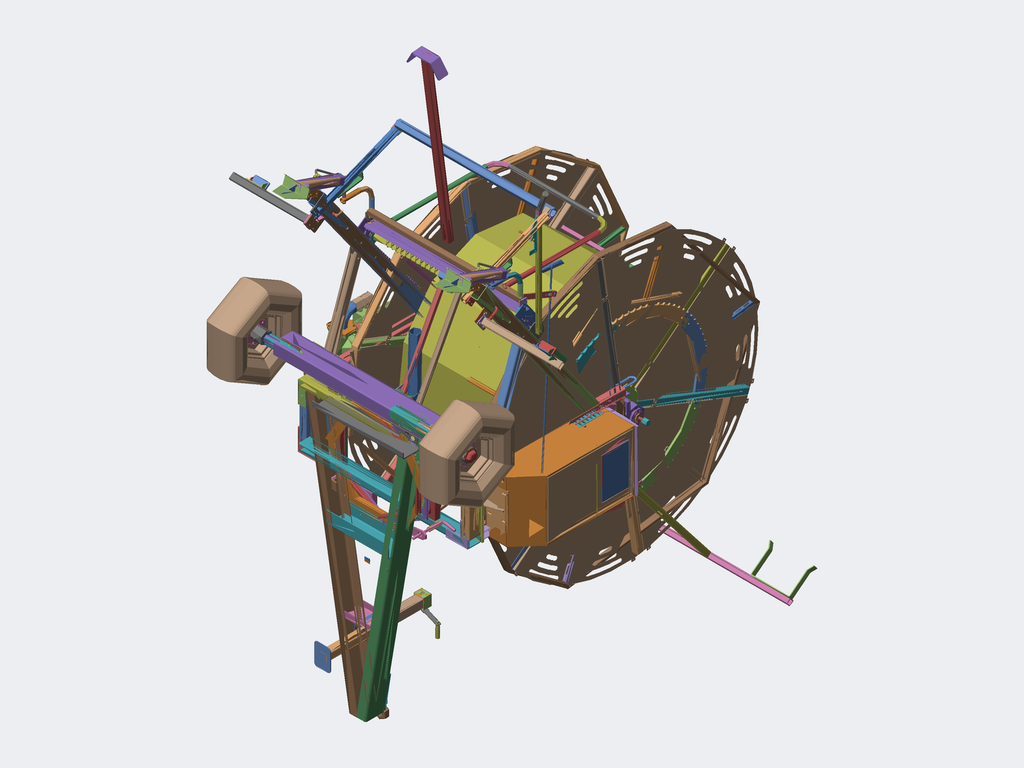Assembly | SolidWorks | 198 different items | 556 placed
Parts list (item | name | quantity | parent item | size | volume | features):
1 | 08B Inner Chain Link | x1 | - | - | - | -
2 | (subassembly) | x1 | - | - | - | features CompositeCurve 2
3 | (subassembly) | x1 | - | - | 42347469 mm3 | features CompositeCurve 25, ReferencePattern 11, InContextFeatHolder 2, MirrorCompFeat 2, LocalCirPattern 1
4 | (subassembly) | x1 | - | 1275 x 1167 x 393.469 mm | 1515109 mm3 | features CompositeCurve 9, ReferencePattern 5, MirrorCompFeat 1
5 | (subassembly) | x1 | - | - | - | features CompositeCurve 14
6 | (subassembly) | x1 | - | 850 x 850 x 62 mm | 6412042 mm3 | features ReferencePattern 139, CompositeCurve 9, LocalCirPattern 1
7 | (subassembly) | x1 | - | 138 x 180 x 325 mm | 523357 mm3 | features CompositeCurve 2
8 | (subassembly) | x1 | - | 105 x 440 x 68.5 mm | 381290 mm3 | features CompositeCurve 20
9 | (subassembly) | x2 | - | - | - | features CompositeCurve 6
10 | (subassembly) | x1 | - | - | - | features CompositeCurve 5
11 | (subassembly) | x2 | - | 84 x 93.542 x 20.19 mm | 15903 mm3 | features CompositeCurve 1
12 | (subassembly) | x1 | - | 1209 x 993.396 x 13.92 mm | 70663 mm3 | features ReferencePattern 244, LocalChainPattern 1
13 | (subassembly) | x1 | - | - | - | -
14 | (subassembly) | x2 | in 20 | 35 x 6.3 x 40 mm | 3119 mm3 | -
15 | (subassembly) | x1 | in 20 | 82.44 x 15.115 x 33.039 mm | 9980 mm3 | features CompositeCurve 1
16 | (subassembly) | x1 | - | 390 x 227.837 x 82 mm | 1530239 mm3 | -
17 | (subassembly) | x1 | - | 520 x 920 x 319.997 mm | 6570455 mm3 | features InContextFeatHolder 2
18 | (subassembly) | x1 | - | 550.016 x 318.498 x 397.435 mm | 1409303 mm3 | features CompositeCurve 37
19 | (subassembly) | x2 | in 17 | 48.002 x 12.05 x 47 mm | 11187 mm3 | features AEMSimFeature 1
20 | (subassembly) | x1 | - | 1370 x 197 x 2359 mm | 12525634 mm3 | features InContextFeatHolder 8, CompositeCurve 2
21 | (subassembly) | x1 | - | 1625 x 1990 x 1408 mm | 21000923 mm3 | features CompositeCurve 16
22 | (subassembly) | x1 | - | 51.4 x 48 x 1470 mm | 137893 mm3 | features CompositeCurve 3
23 | (subassembly) | x2 | - | 710 x 710 x 743.5 mm | 77284937 mm3 | features CompositeCurve 25, Cut 1
24 | (subassembly) | x1 | - | 335.143 x 891.073 x 1473 mm | 5779817 mm3 | features CompositeCurve 45, InContextFeatHolder 1
25 | (subassembly) | x1 | in 24 | 48 x 51.5 x 108 mm | 78961 mm3 | features CompositeCurve 3
26 | - | x1 | in 18 | 140 x 105.523 x 353.223 mm | 225582 mm3 | features BaseBody 9
27 | - | x1 | in 4 | 1275 x 1167 x 350.869 mm | 1494130 mm3 | features ICE 4, Fillet 2, WeldCornerFeat 2, WeldMemberFeat 2, 3DProfileFeature 1, MirrorSolid 1, WeldmentFeature 1
28 | - | x1 | in 22 | 1440 x 10 x 10 mm | 113097 mm3 | features Revolution 1
29 | - | x1 | in 6 | 850 x 850 x 48 mm | 3078442 mm3 | features Cut 1, Extrusion 1, HoleWzd 1, ICE 1, SweepCut 1
30 | - | x1 | in 6 | 850 x 850 x 48 mm | 3032308 mm3 | features ICE 2, Extrusion 1, SweepCut 1
31 | - | x140 | in 6 | 16 x 16 x 16 mm | 2145 mm3 | features Revolution 1
32 | - | x2 | in 9 | 17.852 x 45 x 36.623 mm | 5887 mm3 | features Bending 1, FlatPattern 1, SMBaseFlange 1, SheetMetal 1
33 | - | x1 | - | 87.114 x 117.396 x 10 mm | 59196 mm3 | features Extrusion 1
34 | - | x2 | in 9 | 505 x 200 x 74.971 mm | 438985 mm3 | features ICE 3, EdgeFlange 2, FlatPattern 1, Gusset 1, SMBaseFlange 1, SheetMetal 1, SweepThread 1, WeldMemberFeat 1, WeldmentFeature 1
35 | - | x2 | - | 127.5 x 127.5 x 15 mm | 40689 mm3 | features ICE 1, Sweep 1
36 | - | x1 | in 2 | 81.4 x 88.4 x 66.2 mm | 32314 mm3 | features ICE 3, CornerFeat 1, EdgeFlange 1, Fillet 1, FlatPattern 1, SMBaseFlange 1, SheetMetal 1
37 | - | x2 | in 9 | 390 x 100 x 60 mm | 365741 mm3 | features ICE 3, HoleWzd 1, MirrorSolid 1, WeldMemberFeat 1, WeldmentFeature 1
38 | - | x1 | - | 137.972 x 180 x 185 mm | 377579 mm3 | features Chamfer 1, ICE 1, Revolution 1
39 | - | x1 | - | 180 x 400 x 115 mm | 1229288 mm3 | features ICE 4, Fillet 3, Gusset 2, Extrusion 1, HoleWzd 1
40 | - | x1 | in 7 | 137.972 x 180 x 185 mm | 377579 mm3 | features Chamfer 1, ICE 1, MoveCopyBody 1, Revolution 1
41 | - | x1 | in 2 | 565 x 115 x 75 mm | 595954 mm3 | features ICE 3, WeldMemberFeat 2, EdgeFlange 1, FlatPattern 1, SMBaseFlange 1, SheetMetal 1, WeldmentFeature 1
42 | - | x1 | in 10 | 180 x 60 x 10 mm | 103818 mm3 | features Extrusion 1
43 | - | x1 | in 17 | 55 x 19.5 x 39.375 mm | 9114 mm3 | features ICE 11, Fillet 7, BossThin 2, CutThin 2, LPattern 2, CirPattern 1, Emboss 1, Extrusion 1, MirrorPattern 1, Scale 1
44 | - | x1 | in 10 | 60 x 116.5 x 60 mm | 137866 mm3 | features ICE 3, Fillet 1, Revolution 1
45 | - | x1 | in 10 | 30 x 190 x 28 mm | 58353 mm3 | features Chamfer 1, ICE 1, Revolution 1
46 | - | x2 | in 10 | 14 x 47 x 47 mm | 15915 mm3 | features Revolution 1
47 | - | x1 | in 2 | 5 x 5 x 23 mm | 451.339 mm3 | features Extrusion 1, Fillet 1
48 | - | x1 | in 20 | 604.658 x 439.557 x 2 mm | 390296 mm3 | features Extrusion 1, ICE 1
49 | - | x2 | - | 310 x 184.907 x 93.1 mm | 1419775 mm3 | features ICE 13, Fillet 12, Draft 4, RevCut 2, Revolution 2, 3DProfileFeature 1, Chamfer 1, CirPattern 1, HoleWzd 1, RefAxis 1
50 | - | x2 | in 8 | 52 x 7.4 x 3.7 mm | 537.554 mm3 | features ICE 1, Sweep 1
51 | - | x2 | in 23 | 64 x 9.2 x 4.6 mm | 1032 mm3 | features ICE 1, Sweep 1
52 | - | x1 | in 8 | 40 x 440 x 14 mm | 235600 mm3 | features Extrusion 1, ICE 1
53 | - | x1 | in 8 | 105 x 40 x 40 mm | 52528 mm3 | features HoleWzd 1, ICE 1, WeldMemberFeat 1, WeldmentFeature 1
54 | - | x1 | - | 120.458 x 120.458 x 175 mm | 185173 mm3 | features Chamfer 2, Extrusion 1, ICE 1, LPattern 1, Revolution 1
55 | - | x2 | in 11 | 84 x 93.542 x 20 mm | 12226 mm3 | features ICE 3, Extrusion 1
56 | - | x2 | in 11 | 9 x 9 x 20 mm | 1148 mm3 | features 3DProfileFeature 1, Extrusion 1, HoleWzd 1
57 | - | x2 | in 11 | 17.5 x 9 x 20 mm | 1066 mm3 | features ICE 2, Extrusion 1
58 | - | x1 | - | 81 x 81 x 40.5 mm | 121304 mm3 | features RevCut 2, MoveCopyBody 1, Sweep 1, SweepCut 1
59 | - | x1 | - | - | - | features 3DProfileFeature 4, Helix 1, SweepRefSurface 1
60 | - | x1 | - | 39.501 x 141.742 x 39.499 mm | 29526 mm3 | features 3DProfileFeature 2, Helix 1, Sweep 1
61 | - | x1 | - | 1433 x 80 x 270.762 mm | 1230459 mm3 | features 3DProfileFeature 1, EdgeFlange 1, Fillet 1, FlatPattern 1, HoleWzd 1, SMBaseFlange 1, SheetMetal 1, WeldMemberFeat 1, WeldmentFeature 1
62 | - | x2 | in 10 | 46 x 46 x 1 mm | 1316 mm3 | features Extrusion 1
63 | - | x1 | in 10 | - | - | features ExtendRefSurface 10, ICE 9, OffsetRefSurface 8, TrimRefSurface 6, Fillet 4, ThickenCut 4, SewRefSurface 2, Split 2, Chamfer 1, Helix 1, MirrorPattern 1, Revolution 1, SweepCut 1
64 | - | x1 | in 10 | 418.512 x 837.703 x 220 mm | 967255 mm3 | features ICE 5, Chamfer 4, Extrusion 1, MirrorSolid 1, WeldMemberFeat 1, WeldmentFeature 1
65 | - | x2 | in 21 | 70 x 105 x 12 mm | 65059 mm3 | features Extrusion 1
66 | - | x1 | - | 1270 x 184.784 x 82.347 mm | 924037 mm3 | features ICE 3, SM3dBend 3, Fillet 1, FlatPattern 1, SMBaseFlange 1, SheetMetal 1
67 | - | x1 | in 20 | 25 x 35 x 32 mm | 4524 mm3 | features Extrusion 1, ICE 1
68 | - | x2 | in 9 | 208.199 x 56 x 66 mm | 34151 mm3 | features 3DProfileFeature 2, Sweep 1
69 | - | x1 | in 18 | 132.972 x 76 x 132.966 mm | 175775 mm3 | features Chamfer 1, ICE 1, Revolution 1
70 | - | x1 | in 17 | 520 x 920 x 319.997 mm | 6254954 mm3 | features EdgeFlange 13, ICE 11, FlatPattern 7, SheetMetal 6, SMBaseFlange 5, LPattern 3, Cut 2, Chamfer 1, FormToolInstance 1, MirrorSolid 1, SolidToSheetMetal 1
71 | - | x12 | in 3 | 1022 x 1094 x 15 mm | 731412 mm3 | features SMBaseFlange 8, EdgeFlange 6, ICE 2, BreakCorner 1, FlatPattern 1, SheetMetal 1
72 | - | x1 | - | 1086 x 1346 x 2725 mm | 2854762 mm3 | features 3DProfileFeature 2, FlatPattern 2, ICE 2, MirrorSolid 2, MoveCopyBody 2, Stock 2, MirrorPattern 1, SheetMetal 1, WeldMemberFeat 1, WeldmentFeature 1
73 | - | x1 | - | 2700 x 120 x 40 mm | 1184354 mm3 | features WeldMemberFeat 2, 3DProfileFeature 1, WeldCornerFeat 1, WeldmentFeature 1
74 | - | x1 | - | 115 x 120 x 648 mm | 459448 mm3 | features Gusset 4, Cut 1, Extrusion 1, Fillet 1, FlatPattern 1, ICE 1, SMBaseFlange 1, SheetMetal 1, WeldMemberFeat 1, WeldmentFeature 1
75 | - | x1 | in 25 | 40 x 47.5 x 59 mm | 50942 mm3 | features ICE 3, Extrusion 1, Fillet 1, HoleWzd 1
76 | - | x1 | in 18 | 96 x 70 x 96 mm | 39871 mm3 | features Revolution 1, Shell 1
77 | - | x1 | in 10 | 47 x 47 x 43 mm | 54544 mm3 | features Fillet 3, ICE 3, Chamfer 1, Extrusion 1, HoleWzd 1
78 | - | x1 | in 18 | 29 x 29 x 50 mm | 17318 mm3 | features Extrusion 1
79 | - | x1 | in 15 | 24.5 x 13 x 30 mm | 2874 mm3 | features Extrusion 1, ICE 1
80 | - | x1 | in 24 | 89.972 x 76 x 125.857 mm | 125660 mm3 | features Chamfer 1, Revolution 1, Split 1
81 | - | x1 | in 15 | 70.865 x 12.969 x 30 mm | 5794 mm3 | features ICE 2, Extrusion 1, Fillet 1
82 | - | x1 | in 15 | 11 x 33 x 11 mm | 1312 mm3 | features Revolution 1
83 | - | x1 | - | 158.16 x 158.6 x 7.2 mm | 83678 mm3 | features ICE 5, Revolution 5, CirPattern 3, LPattern 2
84 | - | x1 | in 8 | 88.261 x 91.8 x 14.2 mm | 61120 mm3 | features ICE 5, Revolution 5, CirPattern 3, LPattern 2
85 | - | x1 | in 16 | 227.837 x 280 x 82 mm | 957079 mm3 | features Extrusion 1, Fillet 1, HoleWzd 1, ICE 1
86 | - | x1 | in 16 | 45 x 100 x 290 mm | 523268 mm3 | features ICE 3, Extrusion 1, Fillet 1
87 | - | x1 | in 17 | 440 x 240 x 2 mm | 211121 mm3 | features Cut 1, Extrusion 1
88 | - | x1 | - | 32 x 32 x 55 mm | 17666 mm3 | features Extrusion 1
89 | - | x1 | in 25 | 15 x 15 x 45 mm | 5260 mm3 | features Chamfer 4, ICE 3, Extrusion 1
90 | - | x1 | in 25 | - | - | features ICE 15, RefSurface 4, Revolution 4, BaseBody 1, Chamfer 1
91 | - | x1 | in 24 | 132.972 x 76 x 132.966 mm | 179855 mm3 | features Chamfer 1, Revolution 1
92 | - | x2 | - | 55 x 40 x 210.02 mm | 80598 mm3 | features FlatPattern 1, SM3dBend 1, SMBaseFlange 1, SheetMetal 1
93 | - | x2 | in 2 | 30 x 30 x 8 mm | 2019 mm3 | features ICE 3, Extrusion 1
94 | - | x1 | in 24 | 76 x 76 x 525 mm | 638592 mm3 | features Chamfer 1, Extrusion 1
95 | - | x3 | in 7, 18 | 76 x 76 x 140 mm | 145605 mm3 | features Chamfer 2, Extrusion 1, ICE 1, LPattern 1
96 | - | x1 | in 18 | 75 x 130 x 10 mm | 89834 mm3 | features Extrusion 1
97 | - | x1 | in 21 | 85 x 80 x 10 mm | 64814 mm3 | features Extrusion 1, HoleWzd 1
98 | - | x1 | in 18 | 182 x 76.1 x 76.1 mm | 182460 mm3 | features Chamfer 1, WeldMemberFeat 1, WeldmentFeature 1
99 | - | x1 | in 18 | 211.75 x 403.566 x 147.274 mm | 1044578 mm3 | features MoveCopyBody 11, Stock 10, ICE 6, Chamfer 1, WeldMemberFeat 1, WeldmentFeature 1
100 | - | x1 | in 18 | 110 x 30 x 35 mm | 17166 mm3 | features FlatPattern 1, Jog 1, SMBaseFlange 1, SheetMetal 1
101 | - | x1 | in 18 | 120 x 120 x 80 mm | 384227 mm3 | features ICE 4, Chamfer 1, Extrusion 1
102 | - | x1 | in 18 | 132.972 x 76 x 132.966 mm | 179855 mm3 | features Chamfer 1, Revolution 1
103 | - | x1 | in 24 | 177 x 120 x 80 mm | 437085 mm3 | features ICE 5, Chamfer 3, Cut 1, Extrusion 1
104 | - | x1 | - | 87.114 x 117.396 x 10 mm | 59196 mm3 | features MirrorStock 1
105 | - | x1 | - | 115 x 120 x 648 mm | 459448 mm3 | features MirrorStock 1
106 | - | x1 | in 2 | 28 x 28 x 120.982 mm | 58497 mm3 | features MBimport 1
107 | - | x1 | - | 500 x 710.009 x 320 mm | 1088969 mm3 | features ICE 6, EdgeFlange 4, Fillet 3, Chamfer 2, SMBaseFlange 2, SheetMetal 2, Cut 1, FlatPattern 1, Shell 1
108 | - | x2 | in 19 | 29.75 x 12.05 x 47 mm | 4659 mm3 | features BaseBody 1
109 | - | x2 | in 19 | 29.75 x 12.05 x 47 mm | 6528 mm3 | features BaseBody 1
110 | - | x123 | in 12 | 24.41 x 13.399 x 13.92 mm | 574.494 mm3 | features Boss 2, DeleteBody 1, Extrusion 1, MirrorSolid 1
111 | - | x3 | in 6, 23 | 12.702 x 18 x 11 mm | 1039 mm3 | features ICE 9, Revolution 9, Fillet 2
112 | - | x1 | in 22 | 55 x 48 x 24 mm | 13448 mm3 | features ICE 4, Fillet 2, Revolution 2, Chamfer 1, MirrorSolid 1, RevCut 1, Sweep 1
113 | - | x2 | in 9 | 47.841 x 25 x 47.841 mm | 21610 mm3 | features BaseBody 1
114 | - | x1 | in 10 | 20 x 8 x 7 mm | 1023 mm3 | features Extrusion 1, Fillet 1
115 | - | x2 | in 21 | 12 x 47 x 47 mm | 11391 mm3 | features Revolution 5, CirPattern 2, RefAxis 1, RevCut 1
116 | - | x4 | in 23 | 18 x 80 x 80 mm | 53386 mm3 | features Revolution 5, CirPattern 2, RefAxis 1, RevCut 1
117 | - | x1 | in 21 | 10.9 x 9.44 x 6.4 mm | 370.095 mm3 | features Cut 2, Chamfer 1, Extrusion 1
118 | - | x1 | in 21 | 16 x 11.547 x 10 mm | 685.126 mm3 | features Chamfer 2, RevCut 2, Revolution 2, Extrusion 1, ICE 1
119 | - | x2 | in 10 | 86.4 x 18.475 x 16 mm | 7671 mm3 | features RevCut 3, Extrusion 1, Fillet 1, LPattern 1, Revolution 1
120 | - | x3 | in 22 | 31.4 x 18.475 x 16 mm | 3338 mm3 | features RevCut 3, Extrusion 1, Fillet 1, LPattern 1, Revolution 1
121 | - | x1 | in 17 | - | 5761098 mm3 | features BaseBody 28
122 | - | x2 | in 11 | 44 x 11.547 x 10 mm | 1463 mm3 | features RevCut 3, Extrusion 1, Fillet 1, LPattern 1, Revolution 1
123 | - | x1 | - | 127.5 x 20.785 x 18 mm | 15623 mm3 | features RevCut 3, Extrusion 1, Fillet 1, LPattern 1, Revolution 1
124 | - | x6 | in 4 | 18 x 20.785 x 10.8 mm | 2151 mm3 | features Cut 2, Extrusion 1
125 | - | x6 | in 10, 20 | 24 x 27.713 x 14.8 mm | 5128 mm3 | features Cut 2, Extrusion 1
126 | - | x7 | in 10, 22 | 16 x 18.475 x 8.4 mm | 1366 mm3 | features ICE 2, RevCut 2, Extrusion 1
127 | - | x1 | - | 18 x 20.785 x 10.8 mm | 2103 mm3 | features Cut 2, Chamfer 1, Extrusion 1
128 | - | x1 | in 16 | 52.646 x 60.79 x 34.7 mm | 49893 mm3 | features Cut 3, Chamfer 1, CirPattern 1, Extrusion 1
129 | - | x2 | in 2 | 25.6 x 29.56 x 17 mm | 6436 mm3 | features Cut 2, Chamfer 1, Extrusion 1
130 | - | x2 | in 4 | 18 x 20.785 x 21 mm | 4036 mm3 | features Cut 3, Extrusion 1, Revolution 1
131 | - | x2 | in 10 | 16.182 x 16.166 x 2 mm | 241.9 mm3 | features Extrusion 1
132 | - | x1 | in 2 | 35 x 35 x 19 mm | 13347 mm3 | features ICE 4, Blend 1, Chamfer 1, Extrusion 1
133 | - | x1 | in 10 | 25.172 x 25.146 x 3.2 mm | 909.871 mm3 | features Extrusion 1
134 | - | x2 | in 23 | 85.5 x 83.408 x 2.5 mm | 3180 mm3 | features Extrusion 1
135 | - | x1 | in 10 | 50.5 x 48.578 x 1.5 mm | 759.16 mm3 | features Extrusion 1
136 | - | x2 | in 23 | 36.439 x 36.377 x 6 mm | 3321 mm3 | features Extrusion 1
137 | - | x2 | in 23 | 34.251 x 39.55 x 23.9 mm | 13268 mm3 | features Cut 3, Chamfer 1, CirPattern 1, Extrusion 1
138 | - | x2 | in 10 | 20 x 20 x 2 mm | 455.138 mm3 | features Extrusion 1
139 | - | x5 | in 2, 9 | 24 x 24 x 2.5 mm | 799.143 mm3 | features Extrusion 1
140 | - | x4 | in 8, 10 | 30 x 30 x 3 mm | 1440 mm3 | features Extrusion 1
141 | - | x2 | in 10 | 37 x 37 x 3 mm | 2187 mm3 | features Extrusion 1
142 | - | x2 | in 23 | 44 x 44 x 4 mm | 4119 mm3 | features Extrusion 1
143 | - | x1 | in 3 | 14.048 x 1371 x 1371 mm | 4173248 mm3 | features CirPattern 2, ICE 2, Cut 1, HoleWzd 1, Revolution 1
144 | - | x2 | in 9 | 11 x 18.425 x 12.702 mm | 861.691 mm3 | features BaseBody 1
145 | - | x1 | in 17 | 110 x 39 x 78.75 mm | 72913 mm3 | features ICE 11, Fillet 7, BossThin 2, CutThin 2, LPattern 2, CirPattern 1, Emboss 1, Extrusion 1, MirrorPattern 1
146 | - | x1 | - | - | - | features Sweep 6, Helix 5, 3DProfileFeature 2
147 | - | x1 | - | 379.2 x 630 x 367.794 mm | 25839555 mm3 | features ICE 35, CirPattern 5, Revolution 5, Fillet 3, Blend 2, Chamfer 2, CombineBodies 2, MirrorPattern 1, MirrorSolid 1, MoveFace 1, Scale 1
148 | - | x1 | in 20 | 1370 x 90 x 169.999 mm | 3268075 mm3 | features Cut 2, WeldMemberFeat 2, FlatPattern 1, MirrorSolid 1, SM3dBend 1, SMBaseFlange 1, SheetMetal 1, WeldmentFeature 1
149 | - | x1 | in 20 | 2311 x 160 x 74.999 mm | 3368982 mm3 | features Split 4, Cut 2, 3DProfileFeature 1, FlatPattern 1, Fold 1, HoleWzd 1, SM3dBend 1, SMBaseFlange 1, SheetMetal 1, UnFold 1, WeldmentFeature 1
150 | - | x1 | in 20 | 92 x 68.996 x 44.996 mm | 49140 mm3 | features Fillet 1, FlatPattern 1, SM3dBend 1, SMBaseFlange 1, SheetMetal 1
151 | - | x1 | in 20 | 2311 x 160 x 74.999 mm | 3368985 mm3 | features Split 4, Cut 2, 3DProfileFeature 1, FlatPattern 1, Fold 1, HoleWzd 1, SM3dBend 1, SMBaseFlange 1, SheetMetal 1, UnFold 1, WeldmentFeature 1
152 | - | x1 | in 20 | 750 x 155 x 194.999 mm | 1173169 mm3 | features Cut 1, FlatPattern 1, HoleWzd 1, SM3dBend 1, SMBaseFlange 1, SheetMetal 1, Split 1
153 | - | x1 | in 20 | 300 x 155 x 54.999 mm | 345967 mm3 | features Split 2, FlatPattern 1, HoleWzd 1, SM3dBend 1, SMBaseFlange 1, SheetMetal 1
154 | - | x1 | in 8 | 20 x 58.5 x 20 mm | 12679 mm3 | features Chamfer 1, ICE 1, Revolution 1
155 | - | x1 | in 20 | 510 x 155 x 99.999 mm | 817688 mm3 | features FlatPattern 1, HoleWzd 1, ICE 1, SM3dBend 1, SMBaseFlange 1, SheetMetal 1, Split 1
156 | - | x1 | in 21 | 800 x 480 x 1.5 mm | 561110 mm3 | features FlatPattern 1, ICE 1, SMBaseFlange 1, SheetMetal 1
157 | - | x1 | in 21 | 1815 x 180 x 1367 mm | 6438478 mm3 | features ICE 12, Cut 6, WeldCornerFeat 5, WeldMemberFeat 5, 3DProfileFeature 3, Gusset 3, HoleWzd 3, DeleteBody 2, MirrorSolid 2, MoveCopyBody 2, Extrusion 1, Fillet 1, FlatPattern 1, SM3dBend 1, SMBaseFlange 1, SheetMetal 1, Sweep 1, WeldmentFeature 1
158 | - | x1 | in 21 | 1815 x 315 x 1367 mm | 6905440 mm3 | features ICE 15, Cut 6, WeldCornerFeat 4, WeldMemberFeat 4, 3DProfileFeature 3, Gusset 3, HoleWzd 3, Sweep 2, Extrusion 1, Fillet 1, FlatPattern 1, MirrorSolid 1, MoveCopyBody 1, SM3dBend 1, SMBaseFlange 1, SheetMetal 1, WeldmentFeature 1
159 | - | x2 | - | 1550 x 90 x 50 mm | 1146938 mm3 | features HoleWzd 2, LPattern 1, Split 1, WeldMemberFeat 1, WeldmentFeature 1
160 | - | x1 | - | 1030 x 86.429 x 90 mm | 351764 mm3 | features HoleWzd 2, ICE 1, WeldMemberFeat 1, WeldmentFeature 1
161 | - | x1 | in 3 | 2340 x 2340 x 60 mm | 8212314 mm3 | features WeldMemberFeat 3, ICE 2, 3DProfileFeature 1, Cut 1, WeldmentFeature 1
162 | - | x1 | in 3 | 2340 x 2340 x 85 mm | 8494790 mm3 | features FlatPattern 6, ICE 5, WeldMemberFeat 3, CirPattern 2, HoleWzd 2, 3DProfileFeature 1, EdgeFlange 1, Fillet 1, SMBaseFlange 1, SheetMetal 1, WeldmentFeature 1
163 | - | x1 | - | 1280 x 800 x 70.292 mm | 1562390 mm3 | features 3DProfileFeature 2, HoleWzd 2, ICE 2, MirrorSolid 2, WeldMemberFeat 2, WeldmentFeature 1
164 | - | x1 | in 8 | 20 x 68.5 x 20 mm | 13969 mm3 | features ICE 1, Revolution 1
165 | - | x1 | in 21 | 1400 x 880 x 118 mm | 7030026 mm3 | features ICE 4, HoleWzd 2, WeldMemberFeat 2, LPattern 1, MoveCopyBody 1, WeldmentFeature 1
166 | - | x1 | in 2 | - | - | features ICE 2, Chamfer 1, Extrusion 1, Helix 1, SweepCut 1
167 | - | x1 | - | 93.66 x 68.58 x 50.292 mm | 77419 mm3 | features ICE 4, ConnectionPoint 2, Fillet 2, MoveFace 2, Revolution 2, MoveCopyBody 1, RoutePoint 1, Scale 1
168 | - | x1 | in 18 | 100 x 140 x 44 mm | 86746 mm3 | features ICE 6, Fillet 2, Chamfer 1, Extrusion 1, MirrorPattern 1, Revolution 1
169 | - | x1 | in 2 | 110 x 200 x 40 mm | 43181 mm3 | features ICE 2, Fillet 1, Sweep 1
170 | - | x2 | in 14 | 20.65 x 6.3 x 40 mm | 1684 mm3 | features BaseBody 1
171 | - | x2 | in 14 | 20.65 x 6.3 x 40 mm | 1435 mm3 | features BaseBody 1
172 | - | x2 | in 9 | - | - | features ICE 2, Chamfer 1, Extrusion 1, Helix 1, SweepCut 1
173 | - | x1 | in 22 | 16 x 16 x 60 mm | 5278 mm3 | features Extrusion 1
174 | - | x2 | - | 110 x 260 x 20 mm | 106750 mm3 | features Chamfer 2, Sweep 1
175 | - | x1 | in 2 | 43.5 x 43.5 x 20 mm | 21997 mm3 | features ICE 2, Blend 1, Extrusion 1
176 | - | x2 | in 23 | 264 x 710 x 710 mm | 75274226 mm3 | features Revolution 2, ICE 1
177 | - | x2 | in 23 | 180 x 180 x 130 mm | 680348 mm3 | features ICE 7, HoleWzd 2, Chamfer 1, Extrusion 1
178 | - | x2 | in 23 | 495 x 60 x 60 mm | 418098 mm3 | features Cut 2, WeldMemberFeat 1, WeldmentFeature 1
179 | - | x2 | in 23 | 50 x 50 x 446 mm | 738051 mm3 | features ICE 2, Chamfer 1, Extrusion 1
180 | - | x2 | in 23 | 108 x 30 x 108 mm | 27953 mm3 | features ICE 1, Revolution 1
181 | - | x4 | in 18, 24 | 106 x 11.67 x 106 mm | 13391 mm3 | features Revolution 1
182 | - | x1 | in 24 | 76 x 184.67 x 76 mm | 170240 mm3 | features ICE 2, BlendCut 1, Revolution 1
183 | - | x1 | in 24 | 89 x 89 x 279.1 mm | 698533 mm3 | features Chamfer 2, ICE 2, Extrusion 1
184 | - | x1 | in 25 | 48 x 48 x 10 mm | 16281 mm3 | features Extrusion 1
185 | - | x1 | in 24 | 1176 x 89 x 89 mm | 3262124 mm3 | features ICE 5, 3DProfileFeature 2, Chamfer 2, Cut 1, DelFace 1, DeleteBody 1, HoleWzd 1, RefCurve 1, Revolution 1, Split 1, SurfCut 1
186 | - | x1 | - | - | - | features Fillet 1, MBimport 1
187 | - | x2 | in 23 | 5.21 x 79.5 x 79.5 mm | 14367 mm3 | features Chamfer 2, Revolution 1
188 | - | x1 | in 3 | 1520 x 1520 x 1030 mm | 12689787 mm3 | features WeldMemberFeat 2, CirPattern 1, Cut 1, FlatPattern 1, ICE 1, MirrorSolid 1, MoveCopyBody 1, SMBaseFlange 1, SheetMetal 1, WeldmentFeature 1
189 | - | x1 | in 2 | 30 x 30 x 7 mm | 2499 mm3 | features Extrusion 1, ICE 1
190 | - | x3 | in 2, 9 | 26 x 26 x 11.5 mm | 4545 mm3 | features Extrusion 1, Fillet 1
191 | - | x1 | - | 46.249 x 52.7 x 46.542 mm | 34114 mm3 | features ICE 3, Revolution 2
192 | - | x1 | in 2 | 498.5 x 130 x 180 mm | 585064 mm3 | features ICE 2, HoleWzd 1, WeldMemberFeat 1, WeldmentFeature 1
193 | - | x1 | in 24 | 89 x 89 x 95 mm | 239064 mm3 | features Chamfer 1, Extrusion 1, ICE 1
194 | - | x1 | - | 368.66 x 40 x 234.641 mm | 156675 mm3 | features EdgeFlange 2, FlatPattern 1, SMBaseFlange 1, SheetMetal 1
195 | - | x2 | - | 63 x 17.5 x 3 mm | 910.243 mm3 | features BaseBody 1, ICE 1, Scale 1
196 | - | x1 | - | 780 x 780 x 250 mm | 1146296 mm3 | features WeldCornerFeat 2, WeldMemberFeat 2, 3DProfileFeature 1, Cut 1, HoleWzd 1, MoveCopyBody 1, Split 1, WeldmentFeature 1
197 | - | x1 | in 10 | 88 x 88 x 25.063 mm | 77723 mm3 | features BaseBody 1
198 | GB/T 5786-2000[Hex Head Bolt Fine Thread Full Thread M12x1.5x90] | x1 | - | - | - | -
Mates (type | each side: item.copy, entity, surface, feature), first 400 of 510 lines:
In the top assembly
Width | 178.1 face plane Cold-formed Square Hollow Section gb/t6728-2002 60 X 60 X 4(1) | 178.1 face plane Cold-formed Square Hollow Section gb/t6728-2002 60 X 60 X 4(1) | 148.1 face plane Base-Flange 1 | assembly face
Width | 178.1 face plane Cold-formed Square Hollow Section gb/t6728-2002 60 X 60 X 4(1) | 178.1 face plane Cold-formed Square Hollow Section gb/t6728-2002 60 X 60 X 4(1) | assembly face | 148.1 face plane Base-Flange 1
Coincident | assembly face | 178.1 face
Width | 178.2 face plane Cold-formed Square Hollow Section gb/t6728-2002 60 X 60 X 4(1) | 178.2 face plane Cold-formed Square Hollow Section gb/t6728-2002 60 X 60 X 4(1) | assembly face | 148.1 face plane Base-Flange 1 | 2 times
Coincident | assembly face | 178.2 face
Concentric | 27.1 face cylinder Boss-Extrude 1 | 120.1 face cylinder Boss-Revolve 1
Coincident | 27.1 face plane Boss-Extrude 1 | 120.1 face plane Base-Extrude
Concentric | 120.1 face cylinder Boss-Revolve 1 | 126.1 face cylinder Boss-Extrude 1
Parallel | assembly plane | assembly plane
Concentric | 195.1 face cylinder Import 3 | 35.1 face cylinder Cut-Extrude 1
Concentric | 161.1 face cylinder Boss-Extrude 2 | 183.1 face cylinder Boss-Extrude 1
Coincident | 161.1 face plane Boss-Extrude 2 | 183.1 face plane Cut-Extrude 1
Parallel | 161.1 face plane Cold-formed Square Hollow Section gb/t6728-2002 50 X 50 X 4(1) | 24.1 plane
Parallel | 148.1 face plane Base-Flange 1 | 178.2 face plane Cold-formed Square Hollow Section gb/t6728-2002 60 X 60 X 4(1)
InPlace | 146.1 plane | assembly plane
Coincident | 149.1 face plane Base-Flange 1 | 29.1 face plane Boss-Extrude 2
DistanceDim | 6.1 plane | 148.1 face plane Base-Flange 1
Coincident | 148.1 plane | 6.1 plane
InPlace | 33.1 plane | assembly plane
Coincident | 30.1 face plane Boss-Extrude 1 | 165.1 face plane Cold-formed Rectangular Hollow Section gb/t6728-2002 100X60X4(1)
Concentric | 165.1 edge | 174.1 face cylinder Sweep 1
Coincident | 165.1 face plane Boss-Extrude 3 | 174.1 edge
Concentric | 165.1 edge | 174.2 face cylinder Sweep 1
Coincident | 165.1 face plane Boss-Extrude 3 | 174.2 edge
Concentric | 160.1 face cylinder Dia11.0 (11) DiameterHole 1 | 158.1 face cylinder Boss-Extrude 5
Coincident | 163.1 face plane Cold-formed Round Hollow Section gb/t6728-2002 60 X 4(1) | 157.1 face plane Cold-formed Rectangular Hollow Section gb/t6728-2002 100X60X4(2)
Concentric | 163.1 face cylinder Dia13.0 (13) DiameterHole 1 | 123.1 face cylinder Boss-Revolve 1
Concentric | 123.1 face cylinder Boss-Revolve 1 | 127.1 face cylinder Base-Extrude
Coincident | 163.1 face plane Cold-formed Square Hollow Section gb/t6728-2002 40 X 40 X 3(1) | 127.1 face plane Base-Extrude
Concentric | 163.1 face cylinder Dia13.0 (13) DiameterHole 2 | 157.1 face cylinder Boss-Extrude 5
Concentric | 49.1 edge | 183.1 face cylinder Cut-Extrude 2
Coincident | 49.1 edge | 183.1 face plane Cut-Extrude 2
Coincident | 49.1 face plane Extrude2 | 157.1 face plane Cold-formed Rectangular Hollow Section gb/t6728-2002 80 X 60 X 4(6)
Concentric | 49.1 face cylinder Extrude7 | 157.1 face cylinder Cut-Extrude 1
Coincident | 49.2 face plane Extrude2 | 158.1 face plane Cold-formed Rectangular Hollow Section gb/t6728-2002 80 X 60 X 4(6)
Coincident | 49.2 face plane Revolve2 | 185.1 face plane Cut-Extrude 2
Concentric | 49.2 face cylinder Extrude7 | 158.1 face cylinder Cut-Extrude 1
Concentric | 183.1 face cylinder Cut-Extrude 1 | 83.1 face cylinder Revolve 1
DistanceDim | 83.1 face plane Revolve 1 | 157.1 face plane Cold-formed Rectangular Hollow Section gb/t6728-2002 80 X 60 X 4(6)
Width | 159.1 face plane Cold-formed Rectangular Hollow Section gb/t6728-2002 90 X 50 X 4(1) | 159.1 face plane Cold-formed Rectangular Hollow Section gb/t6728-2002 90 X 50 X 4(1) | 158.1 face plane Cold-formed Rectangular Hollow Section gb/t6728-2002 100X60X4(1) | 158.1 face plane Cold-formed Rectangular Hollow Section gb/t6728-2002 100X60X4(1) | 2 times
Concentric | 159.1 face cylinder Dia20.0 (20) DiameterHole 1 | 158.1 face cylinder Dia20.0 (20) DiameterHole 1
Width | 159.2 face plane Cold-formed Rectangular Hollow Section gb/t6728-2002 90 X 50 X 4(1) | 159.2 face plane Cold-formed Rectangular Hollow Section gb/t6728-2002 90 X 50 X 4(1) | 157.1 face plane Cold-formed Rectangular Hollow Section gb/t6728-2002 100X60X4(2) | 157.1 face plane Cold-formed Rectangular Hollow Section gb/t6728-2002 100X60X4(2) | 2 times
Concentric | 159.2 face cylinder Dia20.0 (20) DiameterHole 1 | 157.1 face cylinder Dia20.0 (20) DiameterHole 1
Concentric | 159.2 face cylinder Dia20.0 (20) DiameterHole 1 | 35.1 face cylinder Sweep 1
Coincident | 35.1 edge | 157.1 face plane Cold-formed Rectangular Hollow Section gb/t6728-2002 100X60X4(2)
Concentric | 115.1 face cylinder Revolve 1 | 63.1 face cylinder Cut-Extrude 6
Coincident | 157.1 face plane Boss-Extrude 3 | 63.1 face plane Split 2
DistanceDim | 55.1 face plane Boss-Extrude 1 | 55.2 face plane Boss-Extrude 1
Coincident | 53.1 face plane Cold-formed Square Hollow Section gb/t6728-2002 40 X 40 X 4(1) | 158.1 face plane Boss-Extrude 1
Perpendicular | 4.1 plane | assembly plane
Concentric | 27.1 face cylinder Boss-Extrude 1 | 120.2 face cylinder Boss-Revolve 1
Coincident | 27.1 face plane Boss-Extrude 1 | 120.2 face plane Base-Extrude
Coincident | 160.1 face plane Cold-formed Square Hollow Section gb/t6728-2002 30 X 30 X 3(1) | 158.1 face plane Boss-Extrude 5
Coincident | assembly face | 84.1 face plane Revolve 1
DistanceDim | 53.1 face plane Cold-formed Square Hollow Section gb/t6728-2002 40 X 40 X 4(1) | 158.1 face plane Boss-Extrude 1
Concentric | 52.1 face cylinder Cut-Extrude 1 | 120.3 face cylinder Boss-Revolve 1
Tangent | 60.1 face surface:4006 Sweep 1 | 158.1 face cylinder Sweep 4
Concentric | 159.1 face cylinder Dia20.0 (20) DiameterHole 1 | 35.2 face cylinder Sweep 1
Coincident | 158.1 face plane Cold-formed Rectangular Hollow Section gb/t6728-2002 100X60X4(1) | 35.2 edge
DistanceDim | 120.3 face plane Base-Extrude | 52.1 face plane Boss-Extrude 1
DistanceDim | assembly face | assembly face | 4 times
Concentric | assembly face | assembly face | 4 times
Coincident | 30.1 plane | 21.1 plane
Coincident | 6.1 plane | 165.1 plane
Coincident | 66.1 face plane Base-Flange 1 | 157.1 face plane Base-Flange 2 | 2 times
DistanceDim | 66.1 vertex | 157.1 face plane Boss-Extrude 3
Coincident | 160.1 face plane Cold-formed Square Hollow Section gb/t6728-2002 30 X 30 X 3(1) | 186.1 face plane FGCT-30-C1.step | 3 times
Coincident | 157.1 face plane Cold-formed Rectangular Hollow Section gb/t6728-2002 80 X 60 X 4(1) | 39.1 face plane Boss-Extrude 2
Width | 39.1 face plane Boss-Extrude 3 | 39.1 face plane Boss-Extrude 1 | 157.1 face plane Cold-formed Rectangular Hollow Section gb/t6728-2002 80 X 60 X 4(1) | 157.1 face plane Cold-formed Rectangular Hollow Section gb/t6728-2002 80 X 60 X 4(1)
DistanceDim | 157.1 face plane Cold-formed Square Hollow Section gb/t6728-2002 60 X 60 X 4(1) | 196.1 face plane Gb/6728-1986 Square Hollow Section 030 X 30 X 2(1)
DistanceDim | 196.1 face plane Gb/6728-1986 Square Hollow Section 030 X 30 X 2(1) | 157.1 face plane Cold-formed Rectangular Hollow Section gb/t6728-2002 80 X 60 X 4(1)
DistanceDim | 157.1 face plane Boss-Extrude 1 | 196.1 face plane Gb/6728-1986 Square Hollow Section 030 X 30 X 2(1)
Coincident | 49.1 face plane Revolve2 | 101.1 face plane Boss-Extrude 1
Coincident | 39.1 face plane Boss-Extrude 1 | 147.1 face plane Boss-Extrude 15
Concentric | 76.1 edge | 54.1 face cylinder Boss-Extrude 1
Width | 39.1 face plane Boss-Extrude 1 | 39.1 face plane Boss-Extrude 1 | 147.1 face plane Boss-Extrude 15 | 147.1 face plane Boss-Extrude 15
Coincident | 158.1 face plane Cold-formed Square Hollow Section gb/t6728-2002 60 X 60 X 4(1) | 70.1 face plane Base-Flange 1
Coincident | 158.1 face plane Cold-formed Square Hollow Section gb/t6728-2002 60 X 60 X 4(1) | 70.1 face plane Edge-Flange 1
DistanceDim | 70.1 face plane Edge-Flange 2 | 158.1 face plane Boss-Extrude 4
Width | 148.1 face plane Cold-formed Square Hollow Section gb/t6728-2002 70 X 70 X 4(1) | 148.1 face plane Cold-formed Square Hollow Section gb/t6728-2002 70 X 70 X 4(1) | 178.2 face plane Cold-formed Square Hollow Section gb/t6728-2002 60 X 60 X 4(1) | 178.2 face plane Cold-formed Square Hollow Section gb/t6728-2002 60 X 60 X 4(1) | 2 times
Width | 148.1 face plane Mirror 1 | 148.1 face plane Mirror 1 | 178.1 face plane Cold-formed Square Hollow Section gb/t6728-2002 60 X 60 X 4(1) | 178.1 face plane Cold-formed Square Hollow Section gb/t6728-2002 60 X 60 X 4(1) | 2 times
Concentric | 159.2 face cylinder Dia14.0 (14) DiameterHole 2 | 37.1 face cylinder Mirror 2
Coincident | 159.2 face plane Split 1 | 37.1 face plane Cold-formed Square Hollow Section gb/t6728-2002 60 X 60 X 4(1)
Coincident | 159.2 face plane Cold-formed Rectangular Hollow Section gb/t6728-2002 90 X 50 X 4(1) | 37.1 face plane Mirror 2
Coincident | 159.1 face plane Split 1 | 37.2 face plane Cold-formed Square Hollow Section gb/t6728-2002 60 X 60 X 4(1)
Width | 159.1 face plane Cold-formed Rectangular Hollow Section gb/t6728-2002 90 X 50 X 4(1) | 159.1 face plane Cold-formed Rectangular Hollow Section gb/t6728-2002 90 X 50 X 4(1) | 37.2 face plane Boss-Extrude 2 | 37.2 face plane Mirror 2
Concentric | 159.1 face cylinder Dia14.0 (14) DiameterHole 2 | 37.2 face cylinder Mirror 2
Concentric | 27.1 face cylinder Boss-Extrude 3 | 158.1 face cylinder Boss-Extrude 6
Concentric | 153.1 face cylinder Dia19.0 (19) DiameterHole 1 | 41.1 face cylinder Cut-Extrude 1 | 2 times
Coincident | 153.1 face plane Base-Flange 1 | 41.1 face plane Hot-rolled Channel gb/t706-2008 6.3(1)
Coincident | 97.1 face plane Boss-Extrude 1 | 96.1 face plane Boss-Extrude 1
Concentric | 99.1 face cylinder 90deg Elbow [1in]14 | assembly face
Coincident | 99.1 face plane 90deg Elbow [1in]14 | assembly face
Parallel | 157.1 face plane Boss-Extrude 1 | assembly face
Concentric | 147.1 face cylinder Revolve 3 | 40.1 face cylinder Boss-Extrude 1
Coincident | 147.1 face plane Revolve 3 | 40.1 face plane Boss-Extrude 1
Coincident | 147.1 face plane Revolve 3 | 38.1 face plane Boss-Extrude 1
Concentric | 38.1 edge | 95.1 face cylinder Boss-Extrude 1
Coincident | 38.1 face plane Revolve 1 | 95.1 face plane Boss-Extrude 1
Coincident | 158.1 face plane Cold-formed Square Hollow Section gb/t6728-2002 60 X 60 X 4(1) | 107.1 face plane Base-Flange 1
Width | 107.1 face plane Edge-Flange 1 | 107.1 face plane Edge-Flange 1 | 158.1 face plane Cold-formed Square Hollow Section gb/t6728-2002 60 X 60 X 4(1) | 158.1 face plane Cold-formed Square Hollow Section gb/t6728-2002 60 X 60 X 4(1)
DistanceDim | 158.1 face plane Boss-Extrude 4 | 107.1 face plane Edge Bend 2
DistanceDim | 27.1 vertex | 157.1 face plane Boss-Extrude 3
DistanceDim | 18.1 plane | 38.1 plane
Concentric | 147.1 face cylinder Revolve 3 | 38.1 face cylinder Boss-Extrude 1
Parallel | 38.1 face plane Boss-Extrude 1 | 95.1 plane
Coincident | 95.2 plane | 95.1 plane
Coincident | 163.1 face plane Cold-formed Square Hollow Section gb/t6728-2002 40 X 40 X 3(1) | 92.1 edge | 2 times
Coincident | 163.1 face plane Cold-formed Square Hollow Section gb/t6728-2002 40 X 40 X 3(1) | 92.1 face plane Base-Flange 1
DistanceDim | 92.1 edge | 163.1 edge
Coincident | 163.1 face plane Cold-formed Square Hollow Section gb/t6728-2002 40 X 40 X 3(1) | 92.2 edge | 2 times
Coincident | 163.1 face plane Cold-formed Square Hollow Section gb/t6728-2002 40 X 40 X 3(1) | 92.2 face plane Base-Flange 1
DistanceDim | 92.2 edge | 163.1 edge
Tangent | 130.1 face sphere Boss-Revolve 1 | 92.2 face plane Base-Flange 1
Concentric | 149.1 face cylinder Cut-Extrude 2 | 85.1 face cylinder Dia18.0 (18) DiameterHole 1
Coincident | 149.1 face plane Base-Flange 1 | 85.1 edge
Coincident | 157.1 face plane Cold-formed Rectangular Hollow Section gb/t6728-2002 80 X 60 X 4(1) | 72.1 face plane Mirror 2
Concentric | 157.1 face cylinder Dia13.0 (13) DiameterHole 5 | 72.1 face cylinder Mirror 2 | 2 times
Coincident | 158.1 face plane Boss-Extrude 7 | 74.1 face plane Boss-Extrude 1
Concentric | 158.1 face cylinder Boss-Extrude 7 | 74.1 face cylinder Boss-Extrude 1 | 2 times
In subassembly 23
Concentric | 116.1 edge | 177.1 edge
Coincident | 177.1 face plane Cut-Extrude 2 | 116.1 face plane Revolve 1
Concentric | 116.2 edge | 116.1 edge
Coincident | 177.1 face plane Cut-Extrude 3 | 116.2 face plane Revolve 1
Concentric | 177.1 edge | 134.1 edge
Coincident | 177.1 face plane Cut-Extrude 7 | 134.1 face plane Base-Extrude
Parallel | 178.3 plane | 23.1 plane
Coincident | 178.3 plane | 23.1 plane | 2 times
DistanceDim | 178.3 face plane Cold-formed Square Hollow Section gb/t6728-2002 60 X 60 X 4(1) | 177.1 face plane Boss-Extrude 1
Concentric | 116.2 edge | 179.1 edge
Concentric | 179.1 edge | 142.1 edge
Concentric | 179.1 edge | 137.1 edge
Concentric | 177.1 face cylinder M10x1.0 Tapped Hole 1 | 111.1 face cone Revolve 1
Tangent | 177.1 face cylinder Boss-Extrude 1 | 111.1 face plane Revolve 1
Concentric | 177.1 edge | 176.1 edge
Coincident | 177.1 face plane Boss-Extrude 2 | 176.1 face plane Boss-Extrude 1
Concentric | 177.1 face cylinder Cut-Extrude 6 | 176.1 face cylinder Boss-Extrude 1
Concentric | 179.1 face cylinder | 187.1 face cylinder Revolve 1
Coincident | 116.1 face plane Revolve 1 | 187.1 face plane Revolve 1
Coincident | 179.1 face plane | 187.1 face plane Revolve 1
Coincident | 179.1 plane | 137.1 plane | 2 times
Concentric | 179.1 face cylinder | 136.1 face cylinder Extrude 1
Coincident | 137.1 face plane Base-Extrude | 136.1 face plane Extrude 1
Coincident | 179.1 face plane | 142.1 face plane Extrude 1
Coincident | 142.1 face plane Extrude 1 | 136.1 face plane Extrude 1
Concentric | 179.1 face cylinder Cut-Extrude 1 | 51.1 face cylinder Sweep 2
DistanceDim | 51.1 edge | 179.1 face cylinder
Concentric | 177.1 edge | 180.1 edge
Coincident | 177.1 face plane Boss-Extrude 1 | 180.1 face plane Revolve 1
Concentric | 177.1 face cylinder M6 Tapped Hole 1 | 180.1 face cylinder Cut-Extrude 1
In subassembly 16
Concentric | 86.1 face cylinder Cut-Extrude 1 | 128.1 face cylinder Base-Extrude
Concentric | 86.1 face cylinder Boss-Extrude 1 | 85.2 face cylinder Boss-Extrude 2
Coincident | 128.1 face plane Base-Extrude | 85.2 face plane Boss-Extrude 2
Parallel | 86.1 face plane Boss-Extrude 2 | 85.2 face plane Boss-Extrude 1
Coincident | 85.2 plane | 16.1 plane | 3 times
Coincident | 86.1 face plane Cut-Extrude 1 | 85.2 face plane Boss-Extrude 2
In subassembly 20
DistanceDim | 149.2 edge | 148.2 edge
Coincident | 148.2 face plane Base-Flange 1 | 149.2 vertex
DistanceDim | 152.1 face plane Base-Flange 1 | 148.2 face plane Base-Flange 1
Width | 152.1 face plane Base-Flange 1 | 152.1 face plane Base-Flange 1 | 148.2 face plane Base-Flange 1 | 148.2 face plane Base-Flange 1
Coincident | 149.2 face plane Base-Flange 1 | 153.2 face plane Base-Flange 1
Width | 153.2 face plane Base-Flange 1 | 153.2 face plane Base-Flange 1 | 148.2 face plane Base-Flange 1 | 148.2 face plane Base-Flange 1
Concentric | 148.2 face cylinder Cut-Extrude 2 | 125.1 face cylinder Base-Extrude
Coincident | 148.2 face plane Base-Flange 1 | 125.1 face plane Base-Extrude
Parallel | 148.2 face plane Base-Flange 1 | 125.1 face plane Base-Extrude
Concentric | 148.2 face cylinder Cut-Extrude 1 | 125.2 face cylinder Base-Extrude
Coincident | 148.2 face plane Base-Flange 1 | 125.2 face plane Base-Extrude
Parallel | 148.2 face plane Base-Flange 1 | 125.2 face plane Base-Extrude
Concentric | 148.2 face cylinder Cut-Extrude 2 | 125.3 face cylinder Base-Extrude
Coincident | 148.2 face plane Base-Flange 1 | 125.3 face plane Base-Extrude
Parallel | 148.2 face plane Base-Flange 1 | 125.3 face plane Base-Extrude
Coincident | 149.2 face plane Base-Flange 1 | 48.1 face plane Boss-Extrude 1
Coincident | 153.2 face plane Base-Flange 1 | 48.1 face plane Boss-Extrude 1
Parallel | 152.1 face plane Base-Flange 1 | 155.1 face plane Base-Flange 1
DistanceDim | 155.1 face plane Base-Flange 1 | 153.2 face plane Base-Flange 1
Width | 155.1 face plane Cut-Extrude 1 | 155.1 face plane Cut-Extrude 1 | 148.2 face plane Base-Flange 1 | 148.2 face plane Base-Flange 1
Coincident | 148.2 face plane Base-Flange 1 | 150.1 face plane Base-Flange 1
Parallel | 153.2 face plane Base-Flange 1 | 79.1 face plane Boss-Extrude 1
Width | 79.1 face plane Boss-Extrude 1 | 79.1 face plane Boss-Extrude 1 | 148.2 face plane Base-Flange 1 | 148.2 face plane Base-Flange 1
DistanceDim | 79.1 vertex | 153.2 edge
Coincident | 153.2 face plane Base-Flange 1 | 67.1 face plane Boss-Extrude 1 | 2 times
Coincident | 153.2 edge | 67.1 edge
DistanceDim | 171.1 vertex | 149.2 edge
Coincident | 149.2 face plane Split 2 | 151.1 face plane Split 3
Coincident | 149.2 face plane Base-Flange 1 | 151.1 face plane Base-Flange 1
DistanceDim | 170.1 vertex | 170.2 vertex
Coincident | 148.2 face plane Mirror 1 | 151.1 edge
Coincident | 148.2 face plane Cold-formed Square Hollow Section gb/t6728-2002 70 X 70 X 4(1) | 149.2 edge
Coincident | 149.2 face plane Split 1 | 151.1 face plane Split 2
Coincident | 152.1 face plane Base-Flange 1 | 151.1 face plane Base-Flange 1
Parallel | 170.2 face plane Import 1 | 170.1 face plane Import 1
Coincident | 171.2 face plane Import 1 | 171.1 face plane Import 1
Parallel | 155.1 face plane Base-Flange 1 | 170.1 face plane Import 1
Coincident | 155.1 face plane Base-Flange 1 | 151.1 face plane Base-Flange 1
Coincident | 155.1 face plane Split 2 | 151.1 face plane Base-Flange 1
Concentric | 148.2 face cylinder Cut-Extrude 1 | 125.4 face cylinder Base-Extrude
Coincident | 148.2 face plane Base-Flange 1 | 125.4 face plane Base-Extrude
In subassembly 14
Concentric | 170.3 face cylinder Import 1 | 171.3 face cylinder Import 1
Coincident | 170.3 face plane Import 1 | 171.3 face plane Import 1
In subassembly 15
Concentric | 79.2 face cylinder Boss-Extrude 1 | 81.1 face cylinder Boss-Extrude 1
Coincident | 79.2 face plane Cut-Extrude 1 | 81.1 edge
Concentric | 79.2 face cylinder Boss-Extrude 1 | 82.1 face cylinder Revolve 1
Coincident | 79.2 face plane Boss-Extrude 1 | 82.1 face plane Revolve 1
LimitPlanarAngleDim | 81.1 face plane Boss-Extrude 1 | 79.2 face plane Boss-Extrude 1
In subassembly 4
Concentric | 27.2 select_type:24 | 124.1 edge
Tangent | 27.2 face cylinder Cold-formed Round Hollow Section gb/t6728-2002 32 X 2(1) | 124.1 face plane Base-Extrude
Coincident | 124.1 edge | 124.2 edge
Coincident | 124.1 face plane Base-Extrude | 124.2 face plane Base-Extrude
Concentric | 124.2 edge | 130.2 edge
Coincident | 124.2 face plane Base-Extrude | 130.2 face plane Base-Extrude
Concentric | 27.2 select_type:24 | 124.3 edge
Tangent | 27.2 face cylinder Cold-formed Round Hollow Section gb/t6728-2002 32 X 2(1) | 124.3 face plane Base-Extrude
In subassembly 3
Concentric | 162.1 edge | 161.2 edge
DistanceDim | 162.1 face plane Cold-formed Square Hollow Section gb/t6728-2002 50 X 50 X 4(1) | 161.2 face plane Cold-formed Square Hollow Section gb/t6728-2002 50 X 50 X 4(1)
Coincident | 162.1 face plane Cold-formed Square Hollow Section gb/t6728-2002 50 X 50 X 4(1) | 161.2 face plane Cold-formed Square Hollow Section gb/t6728-2002 50 X 50 X 4(1)
Concentric | 162.1 face cylinder Boss-Extrude 1 | 143.1 face cylinder Revolve 1
DistanceDim | 143.1 vertex | 162.1 face plane Cold-formed Square Hollow Section gb/t6728-2002 50 X 50 X 4(1)
Coincident | 162.1 face plane Base-Flange 1 | 143.1 face plane CirPattern 3
Coincident | 162.1 face plane Cold-formed Square Hollow Section gb/t6728-2002 50 X 50 X 4(1) | 71.1 face plane Base-Flange 1
Concentric | 162.1 face cylinder Boss-Extrude 1 | 71.1 face cylinder Base-Flange 1
Parallel | 162.1 face plane Cold-formed Square Hollow Section gb/t6728-2002 50 X 50 X 4(1) | 71.1 face plane Edge-Flange 6
Concentric | 162.1 face cylinder Boss-Extrude 1 | 188.1 face cylinder Base-Flange 1
Coincident | 162.1 face plane Cold-formed Square Hollow Section gb/t6728-2002 50 X 50 X 4(1) | 188.1 face plane Body-Move / Copy 2
In subassembly 8
Concentric | 52.2 edge | 53.2 face cylinder Cut-Extrude 1
Coincident | 53.2 face plane Cold-formed Square Hollow Section gb/t6728-2002 40 X 40 X 4(1) | 52.2 face plane Boss-Extrude 1
Coincident | 53.2 face plane Cold-formed Square Hollow Section gb/t6728-2002 40 X 40 X 4(1) | 140.1 face plane Extrude 1
Concentric | 52.2 face cylinder Boss-Extrude 1 | 154.1 face cylinder Revolve 1
Concentric | 154.1 face cylinder Revolve 1 | 84.2 face cylinder Revolve 1
Concentric | 154.1 face cylinder Revolve 1 | 140.2 face cylinder Extrude 1
DistanceDim | 84.2 face plane Revolve 1 | 52.2 face plane Boss-Extrude 1
Coincident | 52.2 face plane Boss-Extrude 1 | 154.1 face plane Revolve 1
Coincident | 154.1 edge | 140.2 face plane Extrude 1
Concentric | 154.1 face cylinder Revolve 1 | 140.3 face cylinder Extrude 1
Coincident | 84.2 face plane Revolve 1 | 140.3 face plane Extrude 1
Concentric | 52.2 face cylinder Boss-Extrude 1 | 164.1 face cylinder Revolve 1
Coincident | 52.2 face plane Boss-Extrude 1 | 164.1 face plane Revolve 1
Concentric | 50.1 face cylinder Sweep 2 | 164.1 face cylinder Cut-Extrude 1
Coincident | 50.1 vertex | 164.1 face cylinder Revolve 1
Concentric | 154.1 face cylinder Cut-Extrude 1 | 50.2 face cylinder Sweep 2
Coincident | 154.1 face cylinder Revolve 1 | 50.2 vertex
Concentric | 140.1 face cylinder Extrude 1 | 164.1 face cylinder Revolve 1
Parallel | 53.2 face plane Cold-formed Square Hollow Section gb/t6728-2002 40 X 40 X 4(1) | 52.2 face plane Boss-Extrude 1
In subassembly 24
Coincident | 183.2 face plane Boss-Extrude 1 | 80.1 face plane Split 2
Parallel | 80.1 plane | 24.2 plane
Concentric | 183.2 face cylinder Boss-Extrude 1 | 185.2 face cylinder Boss-Extrude 3
Parallel | 80.1 plane | 185.2 plane
Concentric | 80.1 edge | 94.1 edge
Coincident | 80.1 face plane Revolve 1 | 94.1 face plane Boss-Extrude 1
Concentric | 94.1 edge | 193.1 edge
Coincident | 94.1 face plane Boss-Extrude 1 | 193.1 face plane Boss-Extrude 1
Concentric | 103.1 edge | 181.1 edge
Coincident | 103.1 face plane Cut-Extrude 3 | 181.1 face plane Revolve 1
Concentric | 103.1 edge | 181.2 edge
Coincident | 103.1 face plane Cut-Extrude 4 | 181.2 face plane Revolve 1
Concentric | 193.1 face cylinder Boss-Extrude 1 | 103.1 edge
Coincident | 193.1 face plane Cut-Extrude 1 | 103.1 face plane Boss-Extrude 1
Concentric | 103.1 edge | 91.1 edge
DistanceDim | 91.1 face plane Revolve 1 | 103.1 face plane Boss-Extrude 1
Coincident | 103.1 plane | 91.1 plane
Parallel | 91.1 plane | 24.2 plane
DistanceDim | 183.2 face plane Boss-Extrude 1 | 185.2 face plane Boss-Extrude 3
Parallel | 182.1 plane | 24.2 plane
Coincident | 91.1 select_type:25 | 182.1 select_type:25
Tangent | 183.2 edge | 80.1 edge
Concentric | 185.2 face cylinder M12 Tapped Hole 1 | 89.1 face cylinder Cut-Extrude 2
Coincident | 185.2 face plane Boss-Extrude 3 | 184.1 face plane Boss-Extrude 1
In subassembly 25
Concentric | 184.2 edge | 89.2 face cylinder Boss-Extrude 1
DistanceDim | 184.2 face plane Boss-Extrude 1 | 89.2 face plane Boss-Extrude 1
Concentric | 89.2 face cylinder Cut-Extrude 1 | 90.1 face cylinder Import 3
Coincident | 89.2 face plane Cut-Extrude 1 | 90.1 face plane Boss-Extrude 2
Concentric | 90.1 face cylinder Import 3 | 75.1 face cylinder Boss-Extrude 3
DistanceDim | 90.1 face plane Boss-Extrude 1 | 75.1 face plane Boss-Extrude 2
Coincident | 75.1 plane | 25.1 plane
In subassembly 11
Concentric | 57.1 face cylinder Cut-Extrude 1 | 122.1 face cylinder Boss-Revolve 1
Coincident | 57.1 face plane Boss-Extrude 2 | 122.1 face plane Base-Extrude
Concentric | 56.1 face cylinder M6 Tapped Hole 1 | 57.1 face cylinder Cut-Extrude 1
Concentric | 56.1 face cylinder Boss-Extrude 1 | 55.3 edge
Coincident | 56.1 face plane Boss-Extrude 1 | 55.3 face plane Boss-Extrude 1
In subassembly 22
Concentric | 173.1 face cylinder Boss-Extrude 1 | 28.1 face cylinder Revolve 1
Tangent | 173.1 face cylinder Boss-Extrude 1 | 120.1 face plane Base-Extrude
Coincident | 120.1 plane | 22.1 plane
DistanceDim | 120.1 face plane Base-Extrude | 173.1 face plane Boss-Extrude 1
Concentric | 28.1 face cylinder Revolve 1 | 126.2 face cylinder Boss-Extrude 1
Concentric | 28.1 face cylinder Revolve 1 | 126.1 face cylinder Boss-Extrude 1
Coincident | 126.2 face plane Boss-Extrude 1 | 126.1 face plane Boss-Extrude 1
DistanceDim | 28.1 face plane Revolve 1 | 173.1 face plane Boss-Extrude 1
Concentric | 28.1 face cylinder Revolve 1 | 112.1 face cylinder Revolve 1
Coincident | 112.1 plane | 22.1 plane
In subassembly 10
Concentric | 63.2 face cylinder Revolve 1 | 197.1 face cylinder VLF02_40_20_D30
Coincident | 63.2 face plane Cut-Extrude 5 | 197.1 face plane VLF02_40_20_D30
Concentric | 63.2 face cylinder Revolve 1 | 64.1 face cylinder Boss-Extrude 1
Coincident | 64.1 face plane Mirror 3 | 45.1 face plane Revolve 1
Concentric | 44.1 face cylinder Cut-Extrude 3 | 46.1 face cylinder Revolve 1
Coincident | 44.1 face plane Revolve 1 | 46.1 face plane Revolve 1
Concentric | 44.1 face cylinder Cut-Extrude 3 | 46.2 face cylinder Revolve 1
Coincident | 44.1 face plane Revolve 1 | 46.2 face plane Revolve 1
Concentric | 45.1 face cylinder Revolve 1 | 46.2 face cylinder Revolve 1
Parallel | 64.1 plane | 42.1 face plane Boss-Extrude 1
Parallel | 64.1 face plane Boss-Extrude 1 | 42.1 face plane Boss-Extrude 1
Concentric | 45.1 face cylinder Revolve 1 | 141.1 face cylinder Extrude 1
Coincident | 64.1 face plane Boss-Extrude 3 | 141.1 face plane Extrude 1
Concentric | 45.1 face cylinder Revolve 1 | 141.2 face cylinder Extrude 1
Coincident | 64.1 face plane Mirror 3 | 141.2 face plane Extrude 1
Width | 44.1 face plane Revolve 1 | 44.1 face plane Revolve 1 | 141.1 face plane Extrude 1 | 141.2 face plane Extrude 1
Concentric | 45.1 face cylinder Revolve 1 | 140.1 face cylinder Extrude 1
Coincident | 64.1 face plane Boss-Extrude 3 | 140.1 face plane Extrude 1
Concentric | 45.1 face cylinder Revolve 1 | 133.1 face cylinder Extrude 1
Coincident | 140.1 face plane Extrude 1 | 133.1 face plane Extrude 1
Concentric | 45.1 face cylinder Revolve 1 | 125.1 face cylinder Base-Extrude
Coincident | 133.1 face plane Extrude 1 | 125.1 face plane Base-Extrude
Concentric | 45.1 face cylinder Revolve 1 | 125.5 face cylinder Base-Extrude
Coincident | 125.1 face plane Base-Extrude | 125.5 face plane Base-Extrude
Tangent | 64.1 face cylinder Cold-formed Round Hollow Section gb/t6728-2002 42.3 X 3(1) | 126.2 face plane Boss-Extrude 1 | 2 times
Concentric | 64.1 face cylinder Cut-Extrude 6 | 119.1 face cylinder Boss-Revolve 1
Tangent | 64.1 face cylinder Cold-formed Round Hollow Section gb/t6728-2002 42.3 X 3(1) | 119.1 face plane Base-Extrude
Concentric | 126.2 face cylinder Boss-Extrude 1 | 119.1 face cylinder Boss-Revolve 1
Coincident | 42.1 face plane Boss-Extrude 1 | 126.2 face plane Boss-Extrude 1
Width | 42.1 face plane Boss-Extrude 1 | 42.1 face plane Boss-Extrude 1 | 64.1 face plane Mirror 3 | 64.1 face plane Boss-Extrude 3
Tangent | 42.1 face plane Boss-Extrude 1 | 119.1 face cylinder Boss-Revolve 1
Concentric | 119.1 face cylinder Boss-Revolve 1 | 131.1 face cylinder Extrude 1
Concentric | 119.1 face cylinder Boss-Revolve 1 | 138.1 face cylinder Extrude 1
Coincident | 42.1 face plane Boss-Extrude 1 | 138.1 face plane Extrude 1
Coincident | 138.1 face plane Extrude 1 | 131.1 face plane Extrude 1
Concentric | 119.1 face cylinder Boss-Revolve 1 | 126.3 face cylinder Boss-Extrude 1
Coincident | 131.1 face plane Extrude 1 | 126.3 face plane Boss-Extrude 1
Concentric | 119.2 face cylinder Boss-Revolve 1 | 126.4 face cylinder Boss-Extrude 1
Concentric | 119.2 face cylinder Boss-Revolve 1 | 131.2 face cylinder Extrude 1
Concentric | 119.2 face cylinder Boss-Revolve 1 | 138.2 face cylinder Extrude 1
Coincident | 138.2 face plane Extrude 1 | 131.2 face plane Extrude 1
Concentric | 119.2 face cylinder Boss-Revolve 1 | 126.5 face cylinder Boss-Extrude 1
Coincident | 131.2 face plane Extrude 1 | 126.5 face plane Boss-Extrude 1
Tangent | 64.1 face cylinder Mirror 3 | 126.4 face plane Boss-Extrude 1 | 2 times
Concentric | 64.1 face cylinder Mirror 3 | 119.2 face cylinder Boss-Revolve 1
Tangent | 64.1 face cylinder Mirror 3 | 119.2 face plane Base-Extrude
Coincident | 42.1 face plane Boss-Extrude 1 | 126.4 face plane Boss-Extrude 1
Tangent | 42.1 face plane Boss-Extrude 1 | 119.2 face cylinder Boss-Revolve 1
Coincident | 42.1 face plane Boss-Extrude 1 | 138.2 face plane Extrude 1
Concentric | 64.1 face cylinder Boss-Extrude 2 | 77.1 face cylinder Boss-Extrude 1
Concentric | 64.1 face cylinder Boss-Extrude 2 | 62.1 face cylinder Boss-Extrude 1
DistanceDim | 64.1 face plane Cut-Extrude 3 | 62.1 face plane Boss-Extrude 1
Concentric | 64.1 face cylinder Boss-Extrude 2 | 62.2 face cylinder Boss-Extrude 1
Coincident | 64.1 face plane Cut-Extrude 3 | 62.2 face plane Boss-Extrude 1
Coincident | 77.1 face plane Boss-Extrude 1 | 62.1 edge
Concentric | 64.1 face cylinder Boss-Extrude 2 | 135.1 face cylinder Base-Extrude
Coincident | 64.1 face plane Cut-Extrude 3 | 135.1 edge
Coincident | 63.2 face plane Cut-Extrude 7 | 114.1 face plane Base-Extrude | 2 times
Concentric | 63.2 face cylinder Cut-Extrude 7 | 114.1 face cylinder Base-Extrude
Coincident | 197.1 face plane VLF02_40_20_D30 | 114.1 face plane Base-Extrude
In subassembly 6
Tangent | 29.2 face torus Cut-Sweep 2 | 31.1 face sphere Revolve 1
Concentric | 29.2 edge | 30.2 edge
DistanceDim | 30.2 face plane Boss-Extrude 1 | 29.2 face plane Boss-Extrude 2
Parallel | 6.2 plane | 111.1 plane
Tangent | 29.2 face cylinder Boss-Extrude 3 | 111.1 face plane Revolve 1
Concentric | 29.2 face cylinder M10x1.0 Tapped Hole 1 | 111.1 face cone Revolve 1
Coincident | 30.2 plane | 6.2 plane
In subassembly 21
Coincident | 165.2 face plane Cold-formed Rectangular Hollow Section gb/t6728-2002 100X60X4(1) | 158.2 face plane Boss-Extrude 1 | 2 times
DistanceDim | 158.2 face plane Boss-Extrude 1 | 165.2 face plane Cold-formed Rectangular Hollow Section gb/t6728-2002 100X60X4(1)
Coincident | 165.2 face plane Cold-formed Rectangular Hollow Section gb/t6728-2002 100X60X4(1) | 157.2 face plane Boss-Extrude 1 | 2 times
Concentric | 157.2 face cylinder Boss-Extrude 4 | 118.1 face cylinder Revolve 1
Coincident | 157.2 face plane Boss-Extrude 4 | 118.1 face plane Boss-Extrude 1
Coincident | 157.2 face plane Boss-Extrude 4 | 117.1 face plane Base-Extrude
Concentric | 118.1 face cylinder Revolve 1 | 117.1 face cylinder Base-Extrude
DistanceDim | 157.2 face plane Boss-Extrude 1 | 165.2 face plane Cold-formed Rectangular Hollow Section gb/t6728-2002 100X60X4(1)
Parallel | 157.2 face plane Cold-formed Rectangular Hollow Section gb/t6728-2002 80 X 60 X 4(1) | 97.2 face plane Boss-Extrude 1
Coincident | 157.2 face plane Cold-formed Rectangular Hollow Section gb/t6728-2002 80 X 60 X 4(6) | 97.2 face plane Boss-Extrude 1 | 2 times
DistanceDim | 97.2 face plane Boss-Extrude 1 | 157.2 face plane Cold-formed Rectangular Hollow Section gb/t6728-2002 80 X 60 X 4(1)
Coincident | 157.2 face plane Boss-Extrude 3 | 65.1 face plane Boss-Extrude 1
Slot | 65.1 face cylinder Boss-Extrude 1 | 157.2 face plane Boss-Extrude 3 | 2 times
Coincident | 158.2 face plane Boss-Extrude 6 | 65.2 face plane Boss-Extrude 1
Slot | 65.2 face cylinder Boss-Extrude 1 | 158.2 face plane Boss-Extrude 6 | 2 times
Concentric | 65.1 face cylinder Boss-Extrude 1 | 115.2 face cylinder Revolve 1
Coincident | 65.1 face plane Boss-Extrude 1 | 115.2 face plane Revolve 1
Concentric | 65.2 face cylinder Boss-Extrude 1 | 115.3 face cylinder Revolve 1
Coincident | 65.2 face plane Boss-Extrude 1 | 115.3 face plane Revolve 1
Coincident | 157.2 face plane Cold-formed Rectangular Hollow Section gb/t6728-2002 80 X 60 X 4(1) | 156.1 face plane Base-Flange 1
Coincident | 157.2 face plane Cold-formed Rectangular Hollow Section gb/t6728-2002 80 X 60 X 4(6) | 156.1 face plane Base-Flange 1
DistanceDim | 156.1 face plane Base-Flange 1 | 157.2 face plane Cold-formed Rectangular Hollow Section gb/t6728-2002 80 X 60 X 4(1)
In subassembly 18
Concentric | 98.1 edge | 102.1 edge
Coincident | 98.1 face plane Welded Steel Pipe gb/t3091-2008 Dia76.1X4.5(1) | 102.1 face plane Revolve 1
Coincident | 102.1 plane | 18.2 plane
Concentric | 98.1 edge | 69.1 edge
Coincident | 98.1 face plane Welded Steel Pipe gb/t3091-2008 Dia76.1X4.5(1) | 69.1 face plane Revolve 1
Coincident | 98.1 plane | 69.1 plane